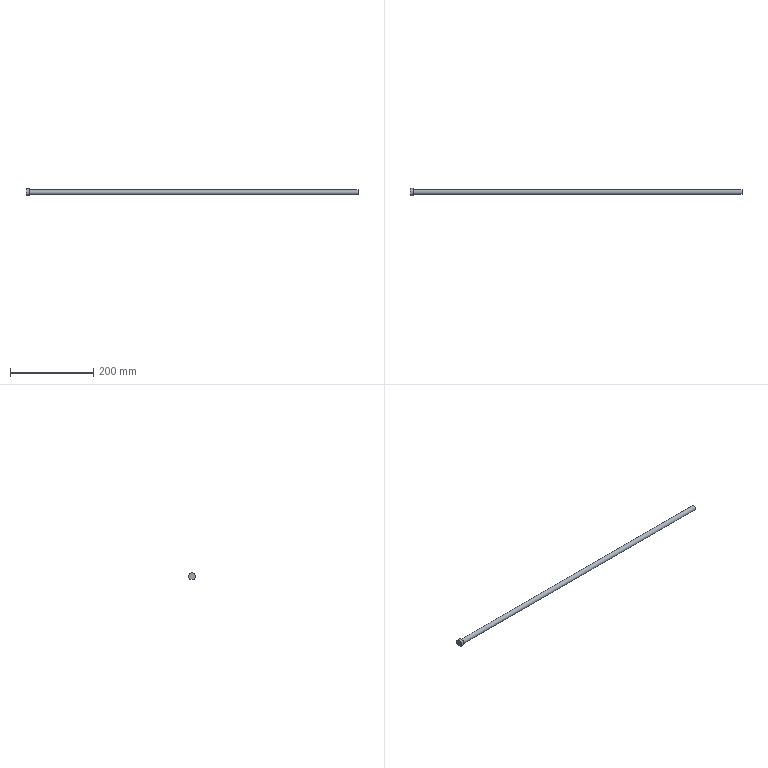Part | STEP file | solid 50 | 1 solid | 6 faces | box 800 x 17 x 15 mm | volume 91269 mm3 | plane 4 | cylinder 2 | commonest cylinder face diameters 12 x1 17 x1